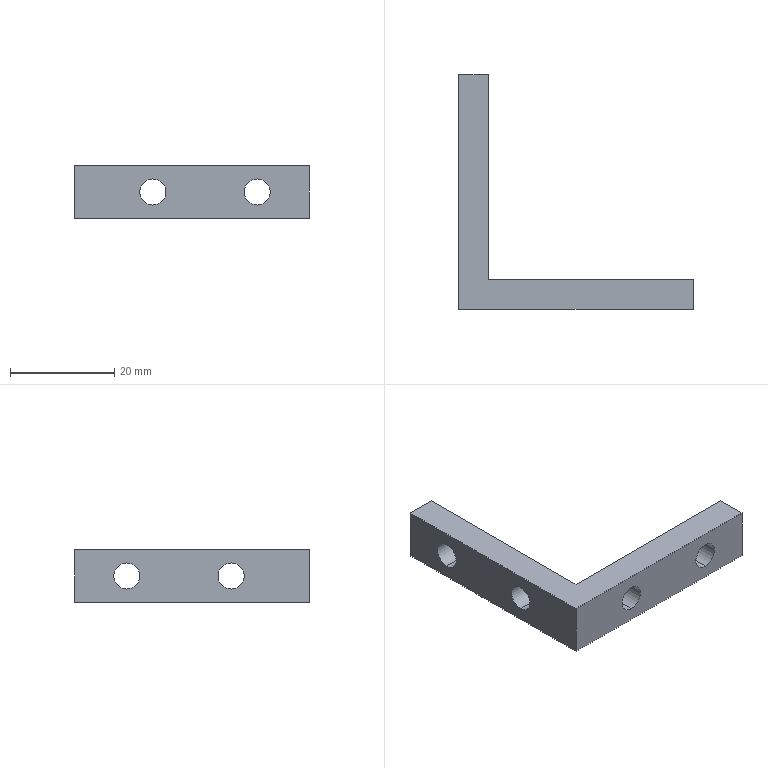Part | NX | features BREP 1 | 1 solid | 16 faces | box 45 x 45 x 10 mm | volume 4357 mm3 | cylinder 8 | plane 8 | commonest cylinder face diameters 5 x8
STEP:
#1=CARTESIAN_POINT('',(15.,5.7,2.5));
#2=VERTEX_POINT('',#1);
#3=CARTESIAN_POINT('',(15.,5.7,-2.5));
#4=VERTEX_POINT('',#3);
#5=CARTESIAN_POINT('',(15.,5.7,0.));
#6=DIRECTION('',(0.,1.,0.));
#7=DIRECTION('',(0.,0.,1.));
#8=AXIS2_PLACEMENT_3D('',#5,#6,#7);
#9=CIRCLE('',#8,2.5);
#10=EDGE_CURVE('',#2,#4,#9,.T.);
#11=ORIENTED_EDGE('',*,*,#10,.T.);
#12=CARTESIAN_POINT('',(15.,0.,-2.5));
#13=VERTEX_POINT('',#12);
#14=CARTESIAN_POINT('',(15.,0.,-2.5));
#15=DIRECTION('',(0.,-1.,0.));
#16=VECTOR('',#15,1000.);
#17=LINE('',#14,#16);
#18=EDGE_CURVE('',#13,#4,#17,.F.);
#19=ORIENTED_EDGE('',*,*,#18,.F.);
#20=CARTESIAN_POINT('',(15.,0.,2.5));
#21=VERTEX_POINT('',#20);
#22=CARTESIAN_POINT('',(15.,0.,0.));
#23=DIRECTION('',(0.,1.,0.));
#24=DIRECTION('',(0.,0.,1.));
#25=AXIS2_PLACEMENT_3D('',#22,#23,#24);
#26=CIRCLE('',#25,2.5);
#27=EDGE_CURVE('',#21,#13,#26,.T.);
#28=ORIENTED_EDGE('',*,*,#27,.F.);
#29=CARTESIAN_POINT('',(15.,0.,2.5));
#30=DIRECTION('',(0.,-1.,0.));
#31=VECTOR('',#30,1000.);
#32=LINE('',#29,#31);
#33=EDGE_CURVE('',#21,#2,#32,.F.);
#34=ORIENTED_EDGE('',*,*,#33,.T.);
#35=EDGE_LOOP('',(#11,#19,#28,#34));
#36=FACE_BOUND('',#35,.T.);
#37=CARTESIAN_POINT('',(15.,0.,0.));
#38=DIRECTION('',(0.,-1.,0.));
#39=DIRECTION('',(0.,0.,1.));
#40=AXIS2_PLACEMENT_3D('',#37,#38,#39);
#41=CYLINDRICAL_SURFACE('',#40,2.5);
#42=ADVANCED_FACE('',(#36),#41,.F.);
#43=CARTESIAN_POINT('',(35.,5.7,2.5));
#44=VERTEX_POINT('',#43);
#45=CARTESIAN_POINT('',(35.,5.7,-2.5));
#46=VERTEX_POINT('',#45);
#47=CARTESIAN_POINT('',(35.,5.7,0.));
#48=DIRECTION('',(0.,1.,0.));
#49=DIRECTION('',(0.,0.,1.));
#50=AXIS2_PLACEMENT_3D('',#47,#48,#49);
#51=CIRCLE('',#50,2.5);
#52=EDGE_CURVE('',#44,#46,#51,.T.);
#53=ORIENTED_EDGE('',*,*,#52,.T.);
#54=CARTESIAN_POINT('',(35.,0.,-2.5));
#55=VERTEX_POINT('',#54);
#56=CARTESIAN_POINT('',(35.,0.,-2.5));
#57=DIRECTION('',(0.,-1.,0.));
#58=VECTOR('',#57,1000.);
#59=LINE('',#56,#58);
#60=EDGE_CURVE('',#55,#46,#59,.F.);
#61=ORIENTED_EDGE('',*,*,#60,.F.);
#62=CARTESIAN_POINT('',(35.,0.,2.5));
#63=VERTEX_POINT('',#62);
#64=CARTESIAN_POINT('',(35.,0.,0.));
#65=DIRECTION('',(0.,1.,0.));
#66=DIRECTION('',(0.,0.,1.));
#67=AXIS2_PLACEMENT_3D('',#64,#65,#66);
#68=CIRCLE('',#67,2.5);
#69=EDGE_CURVE('',#63,#55,#68,.T.);
#70=ORIENTED_EDGE('',*,*,#69,.F.);
#71=CARTESIAN_POINT('',(35.,0.,2.5));
#72=DIRECTION('',(0.,-1.,0.));
#73=VECTOR('',#72,1000.);
#74=LINE('',#71,#73);
#75=EDGE_CURVE('',#63,#44,#74,.F.);
#76=ORIENTED_EDGE('',*,*,#75,.T.);
#77=EDGE_LOOP('',(#53,#61,#70,#76));
#78=FACE_BOUND('',#77,.T.);
#79=CARTESIAN_POINT('',(35.,0.,0.));
#80=DIRECTION('',(0.,-1.,0.));
#81=DIRECTION('',(0.,0.,1.));
#82=AXIS2_PLACEMENT_3D('',#79,#80,#81);
#83=CYLINDRICAL_SURFACE('',#82,2.5);
#84=ADVANCED_FACE('',(#78),#83,.F.);
#85=CARTESIAN_POINT('',(5.7,15.,-2.5));
#86=VERTEX_POINT('',#85);
#87=CARTESIAN_POINT('',(5.7,15.,2.5));
#88=VERTEX_POINT('',#87);
#89=CARTESIAN_POINT('',(5.7,15.,0.));
#90=DIRECTION('',(1.,0.,0.));
#91=DIRECTION('',(0.,-1.,0.));
#92=AXIS2_PLACEMENT_3D('',#89,#90,#91);
#93=CIRCLE('',#92,2.5);
#94=EDGE_CURVE('',#86,#88,#93,.T.);
#95=ORIENTED_EDGE('',*,*,#94,.T.);
#96=CARTESIAN_POINT('',(0.,15.,2.5));
#97=VERTEX_POINT('',#96);
#98=CARTESIAN_POINT('',(0.,15.,2.5));
#99=DIRECTION('',(-1.,0.,0.));
#100=VECTOR('',#99,1000.);
#101=LINE('',#98,#100);
#102=EDGE_CURVE('',#88,#97,#101,.T.);
#103=ORIENTED_EDGE('',*,*,#102,.T.);
#104=CARTESIAN_POINT('',(0.,15.,-2.5));
#105=VERTEX_POINT('',#104);
#106=CARTESIAN_POINT('',(0.,15.,0.));
#107=DIRECTION('',(1.,0.,0.));
#108=DIRECTION('',(0.,0.,-1.));
#109=AXIS2_PLACEMENT_3D('',#106,#107,#108);
#110=CIRCLE('',#109,2.5);
#111=EDGE_CURVE('',#105,#97,#110,.T.);
#112=ORIENTED_EDGE('',*,*,#111,.F.);
#113=CARTESIAN_POINT('',(0.,15.,-2.5));
#114=DIRECTION('',(-1.,0.,0.));
#115=VECTOR('',#114,1000.);
#116=LINE('',#113,#115);
#117=EDGE_CURVE('',#86,#105,#116,.T.);
#118=ORIENTED_EDGE('',*,*,#117,.F.);
#119=EDGE_LOOP('',(#95,#103,#112,#118));
#120=FACE_BOUND('',#119,.T.);
#121=CARTESIAN_POINT('',(0.,15.,0.));
#122=DIRECTION('',(-1.,0.,0.));
#123=DIRECTION('',(0.,0.,-1.));
#124=AXIS2_PLACEMENT_3D('',#121,#122,#123);
#125=CYLINDRICAL_SURFACE('',#124,2.5);
#126=ADVANCED_FACE('',(#120),#125,.F.);
#127=CARTESIAN_POINT('',(5.7,35.,-2.5));
#128=VERTEX_POINT('',#127);
#129=CARTESIAN_POINT('',(5.7,35.,2.5));
#130=VERTEX_POINT('',#129);
#131=CARTESIAN_POINT('',(5.7,35.,0.));
#132=DIRECTION('',(1.,0.,0.));
#133=DIRECTION('',(0.,-1.,0.));
#134=AXIS2_PLACEMENT_3D('',#131,#132,#133);
#135=CIRCLE('',#134,2.5);
#136=EDGE_CURVE('',#128,#130,#135,.T.);
#137=ORIENTED_EDGE('',*,*,#136,.T.);
#138=CARTESIAN_POINT('',(0.,35.,2.5));
#139=VERTEX_POINT('',#138);
#140=CARTESIAN_POINT('',(0.,35.,2.5));
#141=DIRECTION('',(-1.,0.,0.));
#142=VECTOR('',#141,1000.);
#143=LINE('',#140,#142);
#144=EDGE_CURVE('',#130,#139,#143,.T.);
#145=ORIENTED_EDGE('',*,*,#144,.T.);
#146=CARTESIAN_POINT('',(0.,35.,-2.5));
#147=VERTEX_POINT('',#146);
#148=CARTESIAN_POINT('',(0.,35.,0.));
#149=DIRECTION('',(1.,0.,0.));
#150=DIRECTION('',(0.,0.,-1.));
#151=AXIS2_PLACEMENT_3D('',#148,#149,#150);
#152=CIRCLE('',#151,2.5);
#153=EDGE_CURVE('',#147,#139,#152,.T.);
#154=ORIENTED_EDGE('',*,*,#153,.F.);
#155=CARTESIAN_POINT('',(0.,35.,-2.5));
#156=DIRECTION('',(-1.,0.,0.));
#157=VECTOR('',#156,1000.);
#158=LINE('',#155,#157);
#159=EDGE_CURVE('',#128,#147,#158,.T.);
#160=ORIENTED_EDGE('',*,*,#159,.F.);
#161=EDGE_LOOP('',(#137,#145,#154,#160));
#162=FACE_BOUND('',#161,.T.);
#163=CARTESIAN_POINT('',(0.,35.,0.));
#164=DIRECTION('',(-1.,0.,0.));
#165=DIRECTION('',(0.,0.,-1.));
#166=AXIS2_PLACEMENT_3D('',#163,#164,#165);
#167=CYLINDRICAL_SURFACE('',#166,2.5);
#168=ADVANCED_FACE('',(#162),#167,.F.);
#169=CARTESIAN_POINT('',(0.,0.,5.));
#170=VERTEX_POINT('',#169);
#171=CARTESIAN_POINT('',(45.,0.,5.));
#172=VERTEX_POINT('',#171);
#173=CARTESIAN_POINT('',(45.,0.,5.));
#174=DIRECTION('',(1.,0.,0.));
#175=VECTOR('',#174,1000.);
#176=LINE('',#173,#175);
#177=EDGE_CURVE('',#170,#172,#176,.T.);
#178=ORIENTED_EDGE('',*,*,#177,.F.);
#179=CARTESIAN_POINT('',(0.,0.,-5.));
#180=VERTEX_POINT('',#179);
#181=CARTESIAN_POINT('',(0.,0.,-5.));
#182=DIRECTION('',(0.,0.,1.));
#183=VECTOR('',#182,1000.);
#184=LINE('',#181,#183);
#185=EDGE_CURVE('',#180,#170,#184,.T.);
#186=ORIENTED_EDGE('',*,*,#185,.F.);
#187=CARTESIAN_POINT('',(45.,0.,-5.));
#188=VERTEX_POINT('',#187);
#189=CARTESIAN_POINT('',(45.,0.,-5.));
#190=DIRECTION('',(1.,0.,0.));
#191=VECTOR('',#190,1000.);
#192=LINE('',#189,#191);
#193=EDGE_CURVE('',#180,#188,#192,.T.);
#194=ORIENTED_EDGE('',*,*,#193,.T.);
#195=CARTESIAN_POINT('',(45.,0.,-5.));
#196=DIRECTION('',(0.,0.,1.));
#197=VECTOR('',#196,1000.);
#198=LINE('',#195,#197);
#199=EDGE_CURVE('',#188,#172,#198,.T.);
#200=ORIENTED_EDGE('',*,*,#199,.T.);
#201=EDGE_LOOP('',(#178,#186,#194,#200));
#202=FACE_BOUND('',#201,.T.);
#203=ORIENTED_EDGE('',*,*,#27,.T.);
#204=CARTESIAN_POINT('',(15.,0.,0.));
#205=DIRECTION('',(0.,1.,0.));
#206=DIRECTION('',(0.,0.,1.));
#207=AXIS2_PLACEMENT_3D('',#204,#205,#206);
#208=CIRCLE('',#207,2.5);
#209=EDGE_CURVE('',#13,#21,#208,.T.);
#210=ORIENTED_EDGE('',*,*,#209,.T.);
#211=EDGE_LOOP('',(#203,#210));
#212=FACE_BOUND('',#211,.T.);
#213=ORIENTED_EDGE('',*,*,#69,.T.);
#214=CARTESIAN_POINT('',(35.,0.,0.));
#215=DIRECTION('',(0.,1.,0.));
#216=DIRECTION('',(0.,0.,1.));
#217=AXIS2_PLACEMENT_3D('',#214,#215,#216);
#218=CIRCLE('',#217,2.5);
#219=EDGE_CURVE('',#55,#63,#218,.T.);
#220=ORIENTED_EDGE('',*,*,#219,.T.);
#221=EDGE_LOOP('',(#213,#220));
#222=FACE_BOUND('',#221,.T.);
#223=CARTESIAN_POINT('',(45.,0.,-5.));
#224=DIRECTION('',(0.,1.,0.));
#225=DIRECTION('',(1.,0.,0.));
#226=AXIS2_PLACEMENT_3D('',#223,#224,#225);
#227=PLANE('',#226);
#228=ADVANCED_FACE('',(#202,#212,#222),#227,.F.);
#229=CARTESIAN_POINT('',(45.,5.7,5.));
#230=VERTEX_POINT('',#229);
#231=CARTESIAN_POINT('',(45.,5.7,5.));
#232=DIRECTION('',(0.,1.,0.));
#233=VECTOR('',#232,1000.);
#234=LINE('',#231,#233);
#235=EDGE_CURVE('',#172,#230,#234,.T.);
#236=ORIENTED_EDGE('',*,*,#235,.F.);
#237=ORIENTED_EDGE('',*,*,#199,.F.);
#238=CARTESIAN_POINT('',(45.,5.7,-5.));
#239=VERTEX_POINT('',#238);
#240=CARTESIAN_POINT('',(45.,5.7,-5.));
#241=DIRECTION('',(0.,1.,0.));
#242=VECTOR('',#241,1000.);
#243=LINE('',#240,#242);
#244=EDGE_CURVE('',#188,#239,#243,.T.);
#245=ORIENTED_EDGE('',*,*,#244,.T.);
#246=CARTESIAN_POINT('',(45.,5.7,-5.));
#247=DIRECTION('',(0.,0.,1.));
#248=VECTOR('',#247,1000.);
#249=LINE('',#246,#248);
#250=EDGE_CURVE('',#239,#230,#249,.T.);
#251=ORIENTED_EDGE('',*,*,#250,.T.);
#252=EDGE_LOOP('',(#236,#237,#245,#251));
#253=FACE_BOUND('',#252,.T.);
#254=CARTESIAN_POINT('',(45.,5.7,-5.));
#255=DIRECTION('',(-1.,0.,0.));
#256=DIRECTION('',(0.,0.,1.));
#257=AXIS2_PLACEMENT_3D('',#254,#255,#256);
#258=PLANE('',#257);
#259=ADVANCED_FACE('',(#253),#258,.F.);
#260=CARTESIAN_POINT('',(5.7,5.7,5.));
#261=VERTEX_POINT('',#260);
#262=CARTESIAN_POINT('',(5.7,5.7,5.));
#263=DIRECTION('',(-1.,0.,0.));
#264=VECTOR('',#263,1000.);
#265=LINE('',#262,#264);
#266=EDGE_CURVE('',#230,#261,#265,.T.);
#267=ORIENTED_EDGE('',*,*,#266,.F.);
#268=ORIENTED_EDGE('',*,*,#250,.F.);
#269=CARTESIAN_POINT('',(5.7,5.7,-5.));
#270=VERTEX_POINT('',#269);
#271=CARTESIAN_POINT('',(5.7,5.7,-5.));
#272=DIRECTION('',(-1.,0.,0.));
#273=VECTOR('',#272,1000.);
#274=LINE('',#271,#273);
#275=EDGE_CURVE('',#239,#270,#274,.T.);
#276=ORIENTED_EDGE('',*,*,#275,.T.);
#277=CARTESIAN_POINT('',(5.7,5.7,-5.));
#278=DIRECTION('',(0.,0.,1.));
#279=VECTOR('',#278,1000.);
#280=LINE('',#277,#279);
#281=EDGE_CURVE('',#270,#261,#280,.T.);
#282=ORIENTED_EDGE('',*,*,#281,.T.);
#283=EDGE_LOOP('',(#267,#268,#276,#282));
#284=FACE_BOUND('',#283,.T.);
#285=ORIENTED_EDGE('',*,*,#10,.F.);
#286=CARTESIAN_POINT('',(15.,5.7,0.));
#287=DIRECTION('',(0.,1.,0.));
#288=DIRECTION('',(0.,0.,1.));
#289=AXIS2_PLACEMENT_3D('',#286,#287,#288);
#290=CIRCLE('',#289,2.5);
#291=EDGE_CURVE('',#4,#2,#290,.T.);
#292=ORIENTED_EDGE('',*,*,#291,.F.);
#293=EDGE_LOOP('',(#285,#292));
#294=FACE_BOUND('',#293,.T.);
#295=ORIENTED_EDGE('',*,*,#52,.F.);
#296=CARTESIAN_POINT('',(35.,5.7,0.));
#297=DIRECTION('',(0.,1.,0.));
#298=DIRECTION('',(0.,0.,1.));
#299=AXIS2_PLACEMENT_3D('',#296,#297,#298);
#300=CIRCLE('',#299,2.5);
#301=EDGE_CURVE('',#46,#44,#300,.T.);
#302=ORIENTED_EDGE('',*,*,#301,.F.);
#303=EDGE_LOOP('',(#295,#302));
#304=FACE_BOUND('',#303,.T.);
#305=CARTESIAN_POINT('',(5.7,5.7,-5.));
#306=DIRECTION('',(0.,-1.,0.));
#307=DIRECTION('',(0.,0.,-1.));
#308=AXIS2_PLACEMENT_3D('',#305,#306,#307);
#309=PLANE('',#308);
#310=ADVANCED_FACE('',(#284,#294,#304),#309,.F.);
#311=CARTESIAN_POINT('',(5.7,45.,5.));
#312=VERTEX_POINT('',#311);
#313=CARTESIAN_POINT('',(5.7,45.,5.));
#314=DIRECTION('',(0.,1.,0.));
#315=VECTOR('',#314,1000.);
#316=LINE('',#313,#315);
#317=EDGE_CURVE('',#261,#312,#316,.T.);
#318=ORIENTED_EDGE('',*,*,#317,.F.);
#319=ORIENTED_EDGE('',*,*,#281,.F.);
#320=CARTESIAN_POINT('',(5.7,45.,-5.));
#321=VERTEX_POINT('',#320);
#322=CARTESIAN_POINT('',(5.7,45.,-5.));
#323=DIRECTION('',(0.,1.,0.));
#324=VECTOR('',#323,1000.);
#325=LINE('',#322,#324);
#326=EDGE_CURVE('',#270,#321,#325,.T.);
#327=ORIENTED_EDGE('',*,*,#326,.T.);
#328=CARTESIAN_POINT('',(5.7,45.,-5.));
#329=DIRECTION('',(0.,0.,1.));
#330=VECTOR('',#329,1000.);
#331=LINE('',#328,#330);
#332=EDGE_CURVE('',#321,#312,#331,.T.);
#333=ORIENTED_EDGE('',*,*,#332,.T.);
#334=EDGE_LOOP('',(#318,#319,#327,#333));
#335=FACE_BOUND('',#334,.T.);
#336=ORIENTED_EDGE('',*,*,#94,.F.);
#337=CARTESIAN_POINT('',(5.7,15.,0.));
#338=DIRECTION('',(1.,0.,0.));
#339=DIRECTION('',(0.,-1.,0.));
#340=AXIS2_PLACEMENT_3D('',#337,#338,#339);
#341=CIRCLE('',#340,2.5);
#342=EDGE_CURVE('',#88,#86,#341,.T.);
#343=ORIENTED_EDGE('',*,*,#342,.F.);
#344=EDGE_LOOP('',(#336,#343));
#345=FACE_BOUND('',#344,.T.);
#346=ORIENTED_EDGE('',*,*,#136,.F.);
#347=CARTESIAN_POINT('',(5.7,35.,0.));
#348=DIRECTION('',(1.,0.,0.));
#349=DIRECTION('',(0.,-1.,0.));
#350=AXIS2_PLACEMENT_3D('',#347,#348,#349);
#351=CIRCLE('',#350,2.5);
#352=EDGE_CURVE('',#130,#128,#351,.T.);
#353=ORIENTED_EDGE('',*,*,#352,.F.);
#354=EDGE_LOOP('',(#346,#353));
#355=FACE_BOUND('',#354,.T.);
#356=CARTESIAN_POINT('',(5.7,45.,-5.));
#357=DIRECTION('',(-1.,0.,0.));
#358=DIRECTION('',(0.,1.,0.));
#359=AXIS2_PLACEMENT_3D('',#356,#357,#358);
#360=PLANE('',#359);
#361=ADVANCED_FACE('',(#335,#345,#355),#360,.F.);
#362=CARTESIAN_POINT('',(0.,45.,5.));
#363=VERTEX_POINT('',#362);
#364=CARTESIAN_POINT('',(0.,45.,5.));
#365=DIRECTION('',(-1.,0.,0.));
#366=VECTOR('',#365,1000.);
#367=LINE('',#364,#366);
#368=EDGE_CURVE('',#312,#363,#367,.T.);
#369=ORIENTED_EDGE('',*,*,#368,.F.);
#370=ORIENTED_EDGE('',*,*,#332,.F.);
#371=CARTESIAN_POINT('',(0.,45.,-5.));
#372=VERTEX_POINT('',#371);
#373=CARTESIAN_POINT('',(0.,45.,-5.));
#374=DIRECTION('',(-1.,0.,0.));
#375=VECTOR('',#374,1000.);
#376=LINE('',#373,#375);
#377=EDGE_CURVE('',#321,#372,#376,.T.);
#378=ORIENTED_EDGE('',*,*,#377,.T.);
#379=CARTESIAN_POINT('',(0.,45.,-5.));
#380=DIRECTION('',(0.,0.,1.));
#381=VECTOR('',#380,1000.);
#382=LINE('',#379,#381);
#383=EDGE_CURVE('',#372,#363,#382,.T.);
#384=ORIENTED_EDGE('',*,*,#383,.T.);
#385=EDGE_LOOP('',(#369,#370,#378,#384));
#386=FACE_BOUND('',#385,.T.);
#387=CARTESIAN_POINT('',(0.,45.,-5.));
#388=DIRECTION('',(0.,-1.,0.));
#389=DIRECTION('',(0.,0.,-1.));
#390=AXIS2_PLACEMENT_3D('',#387,#388,#389);
#391=PLANE('',#390);
#392=ADVANCED_FACE('',(#386),#391,.F.);
#393=CARTESIAN_POINT('',(0.,0.,5.));
#394=DIRECTION('',(0.,-1.,0.));
#395=VECTOR('',#394,1000.);
#396=LINE('',#393,#395);
#397=EDGE_CURVE('',#363,#170,#396,.T.);
#398=ORIENTED_EDGE('',*,*,#397,.F.);
#399=ORIENTED_EDGE('',*,*,#383,.F.);
#400=CARTESIAN_POINT('',(0.,0.,-5.));
#401=DIRECTION('',(0.,-1.,0.));
#402=VECTOR('',#401,1000.);
#403=LINE('',#400,#402);
#404=EDGE_CURVE('',#372,#180,#403,.T.);
#405=ORIENTED_EDGE('',*,*,#404,.T.);
#406=ORIENTED_EDGE('',*,*,#185,.T.);
#407=EDGE_LOOP('',(#398,#399,#405,#406));
#408=FACE_BOUND('',#407,.T.);
#409=ORIENTED_EDGE('',*,*,#111,.T.);
#410=CARTESIAN_POINT('',(0.,15.,0.));
#411=DIRECTION('',(1.,0.,0.));
#412=DIRECTION('',(0.,0.,-1.));
#413=AXIS2_PLACEMENT_3D('',#410,#411,#412);
#414=CIRCLE('',#413,2.5);
#415=EDGE_CURVE('',#97,#105,#414,.T.);
#416=ORIENTED_EDGE('',*,*,#415,.T.);
#417=EDGE_LOOP('',(#409,#416));
#418=FACE_BOUND('',#417,.T.);
#419=ORIENTED_EDGE('',*,*,#153,.T.);
#420=CARTESIAN_POINT('',(0.,35.,0.));
#421=DIRECTION('',(1.,0.,0.));
#422=DIRECTION('',(0.,0.,-1.));
#423=AXIS2_PLACEMENT_3D('',#420,#421,#422);
#424=CIRCLE('',#423,2.5);
#425=EDGE_CURVE('',#139,#147,#424,.T.);
#426=ORIENTED_EDGE('',*,*,#425,.T.);
#427=EDGE_LOOP('',(#419,#426));
#428=FACE_BOUND('',#427,.T.);
#429=CARTESIAN_POINT('',(0.,0.,-5.));
#430=DIRECTION('',(1.,0.,0.));
#431=DIRECTION('',(0.,1.,0.));
#432=AXIS2_PLACEMENT_3D('',#429,#430,#431);
#433=PLANE('',#432);
#434=ADVANCED_FACE('',(#408,#418,#428),#433,.F.);
#435=ORIENTED_EDGE('',*,*,#193,.F.);
#436=ORIENTED_EDGE('',*,*,#404,.F.);
#437=ORIENTED_EDGE('',*,*,#377,.F.);
#438=ORIENTED_EDGE('',*,*,#326,.F.);
#439=ORIENTED_EDGE('',*,*,#275,.F.);
#440=ORIENTED_EDGE('',*,*,#244,.F.);
#441=EDGE_LOOP('',(#435,#436,#437,#438,#439,#440));
#442=FACE_BOUND('',#441,.T.);
#443=CARTESIAN_POINT('',(0.,0.,-5.));
#444=DIRECTION('',(0.,0.,1.));
#445=DIRECTION('',(1.,0.,0.));
#446=AXIS2_PLACEMENT_3D('',#443,#444,#445);
#447=PLANE('',#446);
#448=ADVANCED_FACE('',(#442),#447,.F.);
#449=ORIENTED_EDGE('',*,*,#177,.T.);
#450=ORIENTED_EDGE('',*,*,#235,.T.);
#451=ORIENTED_EDGE('',*,*,#266,.T.);
#452=ORIENTED_EDGE('',*,*,#317,.T.);
#453=ORIENTED_EDGE('',*,*,#368,.T.);
#454=ORIENTED_EDGE('',*,*,#397,.T.);
#455=EDGE_LOOP('',(#449,#450,#451,#452,#453,#454));
#456=FACE_BOUND('',#455,.T.);
#457=CARTESIAN_POINT('',(0.,0.,5.));
#458=DIRECTION('',(0.,0.,1.));
#459=DIRECTION('',(1.,0.,0.));
#460=AXIS2_PLACEMENT_3D('',#457,#458,#459);
#461=PLANE('',#460);
#462=ADVANCED_FACE('',(#456),#461,.T.);
#463=ORIENTED_EDGE('',*,*,#144,.F.);
#464=ORIENTED_EDGE('',*,*,#352,.T.);
#465=ORIENTED_EDGE('',*,*,#159,.T.);
#466=ORIENTED_EDGE('',*,*,#425,.F.);
#467=EDGE_LOOP('',(#463,#464,#465,#466));
#468=FACE_BOUND('',#467,.T.);
#469=CARTESIAN_POINT('',(0.,35.,0.));
#470=DIRECTION('',(-1.,0.,0.));
#471=DIRECTION('',(0.,0.,-1.));
#472=AXIS2_PLACEMENT_3D('',#469,#470,#471);
#473=CYLINDRICAL_SURFACE('',#472,2.5);
#474=ADVANCED_FACE('',(#468),#473,.F.);
#475=ORIENTED_EDGE('',*,*,#102,.F.);
#476=ORIENTED_EDGE('',*,*,#342,.T.);
#477=ORIENTED_EDGE('',*,*,#117,.T.);
#478=ORIENTED_EDGE('',*,*,#415,.F.);
#479=EDGE_LOOP('',(#475,#476,#477,#478));
#480=FACE_BOUND('',#479,.T.);
#481=CARTESIAN_POINT('',(0.,15.,0.));
#482=DIRECTION('',(-1.,0.,0.));
#483=DIRECTION('',(0.,0.,-1.));
#484=AXIS2_PLACEMENT_3D('',#481,#482,#483);
#485=CYLINDRICAL_SURFACE('',#484,2.5);
#486=ADVANCED_FACE('',(#480),#485,.F.);
#487=ORIENTED_EDGE('',*,*,#60,.T.);
#488=ORIENTED_EDGE('',*,*,#301,.T.);
#489=ORIENTED_EDGE('',*,*,#75,.F.);
#490=ORIENTED_EDGE('',*,*,#219,.F.);
#491=EDGE_LOOP('',(#487,#488,#489,#490));
#492=FACE_BOUND('',#491,.T.);
#493=CARTESIAN_POINT('',(35.,0.,0.));
#494=DIRECTION('',(0.,-1.,0.));
#495=DIRECTION('',(0.,0.,1.));
#496=AXIS2_PLACEMENT_3D('',#493,#494,#495);
#497=CYLINDRICAL_SURFACE('',#496,2.5);
#498=ADVANCED_FACE('',(#492),#497,.F.);
#499=ORIENTED_EDGE('',*,*,#18,.T.);
#500=ORIENTED_EDGE('',*,*,#291,.T.);
#501=ORIENTED_EDGE('',*,*,#33,.F.);
#502=ORIENTED_EDGE('',*,*,#209,.F.);
#503=EDGE_LOOP('',(#499,#500,#501,#502));
#504=FACE_BOUND('',#503,.T.);
#505=CARTESIAN_POINT('',(15.,0.,0.));
#506=DIRECTION('',(0.,-1.,0.));
#507=DIRECTION('',(0.,0.,1.));
#508=AXIS2_PLACEMENT_3D('',#505,#506,#507);
#509=CYLINDRICAL_SURFACE('',#508,2.5);
#510=ADVANCED_FACE('',(#504),#509,.F.);
#511=CLOSED_SHELL('',(#42,#84,#126,#168,#228,#259,#310,#361,#392,#434,#448,#462,#474,#486,#498,#510));
#512=MANIFOLD_SOLID_BREP('',#511);
#513=(LENGTH_UNIT()NAMED_UNIT(*)SI_UNIT(.MILLI.,.METRE.));
#514=UNCERTAINTY_MEASURE_WITH_UNIT(LENGTH_MEASURE(0.00001),#513,'','');
#515=(NAMED_UNIT(*)PLANE_ANGLE_UNIT()SI_UNIT($,.RADIAN.));
#516=(NAMED_UNIT(*)SI_UNIT($,.STERADIAN.)SOLID_ANGLE_UNIT());
#517=(GEOMETRIC_REPRESENTATION_CONTEXT(3)GLOBAL_UNCERTAINTY_ASSIGNED_CONTEXT((#514))GLOBAL_UNIT_ASSIGNED_CONTEXT((#513,#515,#516))REPRESENTATION_CONTEXT('',''));
#518=ADVANCED_BREP_SHAPE_REPRESENTATION('',(#512),#517);